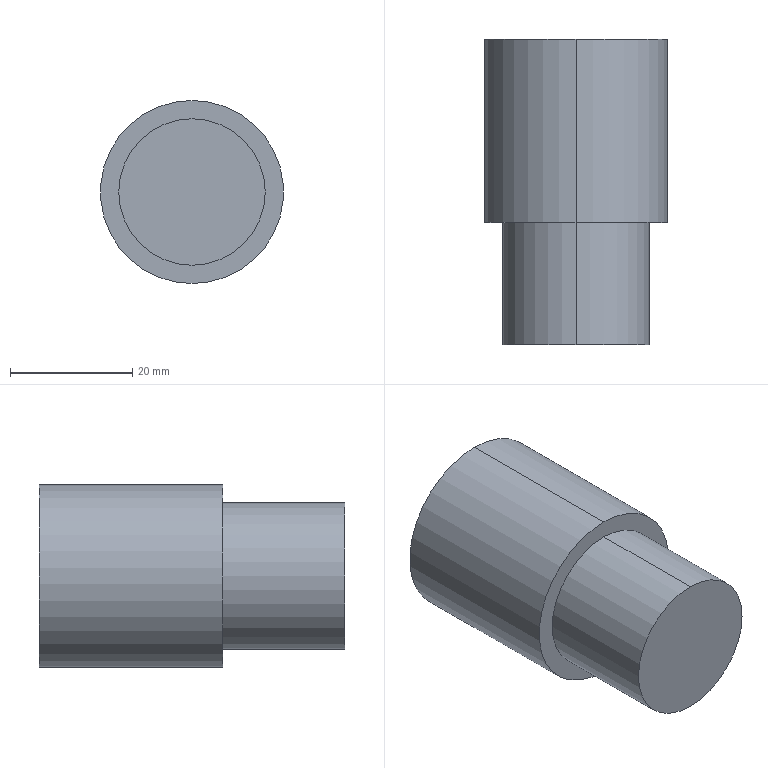Part | 1 solid | 13 faces | box 30 x 50 x 30 mm | volume 20948 mm3 | cylinder 8 | plane 5 | commonest cylinder face diameters 18 x2 20 x2 24 x2 30 x2
STEP:
#1=CARTESIAN_POINT('',(0.,-20.,-12.));
#2=VERTEX_POINT('',#1);
#3=CARTESIAN_POINT('',(0.,-20.,12.));
#4=VERTEX_POINT('',#3);
#5=CARTESIAN_POINT('',(0.,-20.,0.));
#6=DIRECTION('',(0.,-1.,0.));
#7=DIRECTION('',(0.,0.,-1.));
#8=AXIS2_PLACEMENT_3D('',#5,#6,#7);
#9=CIRCLE('',#8,12.);
#10=EDGE_CURVE('',#2,#4,#9,.T.);
#11=ORIENTED_EDGE('',*,*,#10,.F.);
#12=CARTESIAN_POINT('',(0.,0.,-12.));
#13=VERTEX_POINT('',#12);
#14=CARTESIAN_POINT('',(0.,-20.,-12.));
#15=DIRECTION('',(0.,1.,0.));
#16=VECTOR('',#15,1000.);
#17=LINE('',#14,#16);
#18=EDGE_CURVE('',#2,#13,#17,.T.);
#19=ORIENTED_EDGE('',*,*,#18,.T.);
#20=CARTESIAN_POINT('',(0.,0.,12.));
#21=VERTEX_POINT('',#20);
#22=CARTESIAN_POINT('',(0.,0.,0.));
#23=DIRECTION('',(0.,-1.,0.));
#24=DIRECTION('',(0.,0.,-1.));
#25=AXIS2_PLACEMENT_3D('',#22,#23,#24);
#26=CIRCLE('',#25,12.);
#27=EDGE_CURVE('',#13,#21,#26,.T.);
#28=ORIENTED_EDGE('',*,*,#27,.T.);
#29=CARTESIAN_POINT('',(0.,-20.,12.));
#30=DIRECTION('',(0.,1.,0.));
#31=VECTOR('',#30,1000.);
#32=LINE('',#29,#31);
#33=EDGE_CURVE('',#4,#21,#32,.T.);
#34=ORIENTED_EDGE('',*,*,#33,.F.);
#35=EDGE_LOOP('',(#11,#19,#28,#34));
#36=FACE_OUTER_BOUND('',#35,.T.);
#37=CARTESIAN_POINT('',(0.,-20.,0.));
#38=DIRECTION('',(0.,1.,0.));
#39=DIRECTION('',(0.,0.,1.));
#40=AXIS2_PLACEMENT_3D('',#37,#38,#39);
#41=CYLINDRICAL_SURFACE('',#40,12.);
#42=ADVANCED_FACE('',(#36),#41,.T.);
#43=CARTESIAN_POINT('',(0.,30.,15.));
#44=VERTEX_POINT('',#43);
#45=CARTESIAN_POINT('',(0.,30.,-15.));
#46=VERTEX_POINT('',#45);
#47=CARTESIAN_POINT('',(0.,30.,0.));
#48=DIRECTION('',(0.,1.,0.));
#49=DIRECTION('',(0.,0.,1.));
#50=AXIS2_PLACEMENT_3D('',#47,#48,#49);
#51=CIRCLE('',#50,15.);
#52=EDGE_CURVE('',#44,#46,#51,.T.);
#53=ORIENTED_EDGE('',*,*,#52,.F.);
#54=CARTESIAN_POINT('',(0.,0.,15.));
#55=VERTEX_POINT('',#54);
#56=CARTESIAN_POINT('',(0.,30.,15.));
#57=DIRECTION('',(0.,-1.,0.));
#58=VECTOR('',#57,1000.);
#59=LINE('',#56,#58);
#60=EDGE_CURVE('',#44,#55,#59,.T.);
#61=ORIENTED_EDGE('',*,*,#60,.T.);
#62=CARTESIAN_POINT('',(0.,0.,-15.));
#63=VERTEX_POINT('',#62);
#64=CARTESIAN_POINT('',(0.,0.,0.));
#65=DIRECTION('',(0.,1.,0.));
#66=DIRECTION('',(0.,0.,1.));
#67=AXIS2_PLACEMENT_3D('',#64,#65,#66);
#68=CIRCLE('',#67,15.);
#69=EDGE_CURVE('',#55,#63,#68,.T.);
#70=ORIENTED_EDGE('',*,*,#69,.T.);
#71=CARTESIAN_POINT('',(0.,30.,-15.));
#72=DIRECTION('',(0.,-1.,0.));
#73=VECTOR('',#72,1000.);
#74=LINE('',#71,#73);
#75=EDGE_CURVE('',#46,#63,#74,.T.);
#76=ORIENTED_EDGE('',*,*,#75,.F.);
#77=EDGE_LOOP('',(#53,#61,#70,#76));
#78=FACE_OUTER_BOUND('',#77,.T.);
#79=CARTESIAN_POINT('',(0.,30.,0.));
#80=DIRECTION('',(0.,-1.,0.));
#81=DIRECTION('',(0.,0.,-1.));
#82=AXIS2_PLACEMENT_3D('',#79,#80,#81);
#83=CYLINDRICAL_SURFACE('',#82,15.);
#84=ADVANCED_FACE('',(#78),#83,.T.);
#85=CARTESIAN_POINT('',(0.,28.,-9.));
#86=VERTEX_POINT('',#85);
#87=CARTESIAN_POINT('',(0.,28.,9.));
#88=VERTEX_POINT('',#87);
#89=CARTESIAN_POINT('',(0.,28.,0.));
#90=DIRECTION('',(0.,1.,0.));
#91=DIRECTION('',(0.,0.,1.));
#92=AXIS2_PLACEMENT_3D('',#89,#90,#91);
#93=CIRCLE('',#92,9.);
#94=EDGE_CURVE('',#86,#88,#93,.T.);
#95=ORIENTED_EDGE('',*,*,#94,.F.);
#96=CARTESIAN_POINT('',(0.,30.,-9.));
#97=VERTEX_POINT('',#96);
#98=CARTESIAN_POINT('',(0.,25.,-9.));
#99=DIRECTION('',(0.,1.,0.));
#100=VECTOR('',#99,1000.);
#101=LINE('',#98,#100);
#102=EDGE_CURVE('',#86,#97,#101,.T.);
#103=ORIENTED_EDGE('',*,*,#102,.T.);
#104=CARTESIAN_POINT('',(0.,30.,9.));
#105=VERTEX_POINT('',#104);
#106=CARTESIAN_POINT('',(0.,30.,0.));
#107=DIRECTION('',(0.,1.,0.));
#108=DIRECTION('',(0.,0.,1.));
#109=AXIS2_PLACEMENT_3D('',#106,#107,#108);
#110=CIRCLE('',#109,9.);
#111=EDGE_CURVE('',#97,#105,#110,.T.);
#112=ORIENTED_EDGE('',*,*,#111,.T.);
#113=CARTESIAN_POINT('',(0.,25.,9.));
#114=DIRECTION('',(0.,1.,0.));
#115=VECTOR('',#114,1000.);
#116=LINE('',#113,#115);
#117=EDGE_CURVE('',#88,#105,#116,.T.);
#118=ORIENTED_EDGE('',*,*,#117,.F.);
#119=EDGE_LOOP('',(#95,#103,#112,#118));
#120=FACE_OUTER_BOUND('',#119,.T.);
#121=CARTESIAN_POINT('',(0.,25.,0.));
#122=DIRECTION('',(0.,1.,0.));
#123=DIRECTION('',(0.,0.,1.));
#124=AXIS2_PLACEMENT_3D('',#121,#122,#123);
#125=CYLINDRICAL_SURFACE('',#124,9.);
#126=ADVANCED_FACE('',(#120),#125,.F.);
#127=CARTESIAN_POINT('',(0.,0.,-10.));
#128=VERTEX_POINT('',#127);
#129=CARTESIAN_POINT('',(0.,0.,10.));
#130=VERTEX_POINT('',#129);
#131=CARTESIAN_POINT('',(0.,0.,0.));
#132=DIRECTION('',(0.,1.,0.));
#133=DIRECTION('',(0.,0.,1.));
#134=AXIS2_PLACEMENT_3D('',#131,#132,#133);
#135=CIRCLE('',#134,10.);
#136=EDGE_CURVE('',#128,#130,#135,.T.);
#137=ORIENTED_EDGE('',*,*,#136,.F.);
#138=CARTESIAN_POINT('',(0.,28.,-10.));
#139=VERTEX_POINT('',#138);
#140=CARTESIAN_POINT('',(0.,0.,-10.));
#141=DIRECTION('',(0.,1.,0.));
#142=VECTOR('',#141,1000.);
#143=LINE('',#140,#142);
#144=EDGE_CURVE('',#128,#139,#143,.T.);
#145=ORIENTED_EDGE('',*,*,#144,.T.);
#146=CARTESIAN_POINT('',(0.,28.,10.));
#147=VERTEX_POINT('',#146);
#148=CARTESIAN_POINT('',(0.,28.,0.));
#149=DIRECTION('',(0.,1.,0.));
#150=DIRECTION('',(0.,0.,1.));
#151=AXIS2_PLACEMENT_3D('',#148,#149,#150);
#152=CIRCLE('',#151,10.);
#153=EDGE_CURVE('',#139,#147,#152,.T.);
#154=ORIENTED_EDGE('',*,*,#153,.T.);
#155=CARTESIAN_POINT('',(0.,0.,10.));
#156=DIRECTION('',(0.,1.,0.));
#157=VECTOR('',#156,1000.);
#158=LINE('',#155,#157);
#159=EDGE_CURVE('',#130,#147,#158,.T.);
#160=ORIENTED_EDGE('',*,*,#159,.F.);
#161=EDGE_LOOP('',(#137,#145,#154,#160));
#162=FACE_OUTER_BOUND('',#161,.T.);
#163=CARTESIAN_POINT('',(0.,0.,0.));
#164=DIRECTION('',(0.,1.,0.));
#165=DIRECTION('',(0.,0.,1.));
#166=AXIS2_PLACEMENT_3D('',#163,#164,#165);
#167=CYLINDRICAL_SURFACE('',#166,10.);
#168=ADVANCED_FACE('',(#162),#167,.F.);
#169=ORIENTED_EDGE('',*,*,#144,.F.);
#170=CARTESIAN_POINT('',(0.,0.,0.));
#171=DIRECTION('',(0.,1.,0.));
#172=DIRECTION('',(0.,0.,1.));
#173=AXIS2_PLACEMENT_3D('',#170,#171,#172);
#174=CIRCLE('',#173,10.);
#175=EDGE_CURVE('',#130,#128,#174,.T.);
#176=ORIENTED_EDGE('',*,*,#175,.F.);
#177=ORIENTED_EDGE('',*,*,#159,.T.);
#178=CARTESIAN_POINT('',(0.,28.,0.));
#179=DIRECTION('',(0.,1.,0.));
#180=DIRECTION('',(0.,0.,1.));
#181=AXIS2_PLACEMENT_3D('',#178,#179,#180);
#182=CIRCLE('',#181,10.);
#183=EDGE_CURVE('',#147,#139,#182,.T.);
#184=ORIENTED_EDGE('',*,*,#183,.T.);
#185=EDGE_LOOP('',(#169,#176,#177,#184));
#186=FACE_OUTER_BOUND('',#185,.T.);
#187=CARTESIAN_POINT('',(0.,0.,0.));
#188=DIRECTION('',(0.,1.,0.));
#189=DIRECTION('',(0.,0.,1.));
#190=AXIS2_PLACEMENT_3D('',#187,#188,#189);
#191=CYLINDRICAL_SURFACE('',#190,10.);
#192=ADVANCED_FACE('',(#186),#191,.F.);
#193=ORIENTED_EDGE('',*,*,#175,.T.);
#194=ORIENTED_EDGE('',*,*,#136,.T.);
#195=EDGE_LOOP('',(#193,#194));
#196=FACE_OUTER_BOUND('',#195,.T.);
#197=CARTESIAN_POINT('',(0.,0.,0.));
#198=DIRECTION('',(0.,1.,0.));
#199=DIRECTION('',(0.,0.,1.));
#200=AXIS2_PLACEMENT_3D('',#197,#198,#199);
#201=PLANE('',#200);
#202=ADVANCED_FACE('',(#196),#201,.T.);
#203=CARTESIAN_POINT('',(0.,28.,0.));
#204=DIRECTION('',(0.,1.,0.));
#205=DIRECTION('',(0.,0.,1.));
#206=AXIS2_PLACEMENT_3D('',#203,#204,#205);
#207=CIRCLE('',#206,9.);
#208=EDGE_CURVE('',#88,#86,#207,.T.);
#209=ORIENTED_EDGE('',*,*,#208,.T.);
#210=ORIENTED_EDGE('',*,*,#94,.T.);
#211=EDGE_LOOP('',(#209,#210));
#212=FACE_BOUND('',#211,.T.);
#213=ORIENTED_EDGE('',*,*,#183,.F.);
#214=ORIENTED_EDGE('',*,*,#153,.F.);
#215=EDGE_LOOP('',(#213,#214));
#216=FACE_OUTER_BOUND('',#215,.T.);
#217=CARTESIAN_POINT('',(0.,28.,0.));
#218=DIRECTION('',(0.,1.,0.));
#219=DIRECTION('',(0.,0.,1.));
#220=AXIS2_PLACEMENT_3D('',#217,#218,#219);
#221=PLANE('',#220);
#222=ADVANCED_FACE('',(#212,#216),#221,.F.);
#223=ORIENTED_EDGE('',*,*,#102,.F.);
#224=ORIENTED_EDGE('',*,*,#208,.F.);
#225=ORIENTED_EDGE('',*,*,#117,.T.);
#226=CARTESIAN_POINT('',(0.,30.,0.));
#227=DIRECTION('',(0.,1.,0.));
#228=DIRECTION('',(0.,0.,1.));
#229=AXIS2_PLACEMENT_3D('',#226,#227,#228);
#230=CIRCLE('',#229,9.);
#231=EDGE_CURVE('',#105,#97,#230,.T.);
#232=ORIENTED_EDGE('',*,*,#231,.T.);
#233=EDGE_LOOP('',(#223,#224,#225,#232));
#234=FACE_OUTER_BOUND('',#233,.T.);
#235=CARTESIAN_POINT('',(0.,25.,0.));
#236=DIRECTION('',(0.,1.,0.));
#237=DIRECTION('',(0.,0.,1.));
#238=AXIS2_PLACEMENT_3D('',#235,#236,#237);
#239=CYLINDRICAL_SURFACE('',#238,9.);
#240=ADVANCED_FACE('',(#234),#239,.F.);
#241=ORIENTED_EDGE('',*,*,#60,.F.);
#242=CARTESIAN_POINT('',(0.,30.,0.));
#243=DIRECTION('',(0.,1.,0.));
#244=DIRECTION('',(0.,0.,1.));
#245=AXIS2_PLACEMENT_3D('',#242,#243,#244);
#246=CIRCLE('',#245,15.);
#247=EDGE_CURVE('',#46,#44,#246,.T.);
#248=ORIENTED_EDGE('',*,*,#247,.F.);
#249=ORIENTED_EDGE('',*,*,#75,.T.);
#250=CARTESIAN_POINT('',(0.,0.,0.));
#251=DIRECTION('',(0.,1.,0.));
#252=DIRECTION('',(0.,0.,1.));
#253=AXIS2_PLACEMENT_3D('',#250,#251,#252);
#254=CIRCLE('',#253,15.);
#255=EDGE_CURVE('',#63,#55,#254,.T.);
#256=ORIENTED_EDGE('',*,*,#255,.T.);
#257=EDGE_LOOP('',(#241,#248,#249,#256));
#258=FACE_OUTER_BOUND('',#257,.T.);
#259=CARTESIAN_POINT('',(0.,30.,0.));
#260=DIRECTION('',(0.,-1.,0.));
#261=DIRECTION('',(0.,0.,-1.));
#262=AXIS2_PLACEMENT_3D('',#259,#260,#261);
#263=CYLINDRICAL_SURFACE('',#262,15.);
#264=ADVANCED_FACE('',(#258),#263,.T.);
#265=ORIENTED_EDGE('',*,*,#231,.F.);
#266=ORIENTED_EDGE('',*,*,#111,.F.);
#267=EDGE_LOOP('',(#265,#266));
#268=FACE_BOUND('',#267,.T.);
#269=ORIENTED_EDGE('',*,*,#247,.T.);
#270=ORIENTED_EDGE('',*,*,#52,.T.);
#271=EDGE_LOOP('',(#269,#270));
#272=FACE_OUTER_BOUND('',#271,.T.);
#273=CARTESIAN_POINT('',(0.,30.,0.));
#274=DIRECTION('',(0.,1.,0.));
#275=DIRECTION('',(0.,0.,1.));
#276=AXIS2_PLACEMENT_3D('',#273,#274,#275);
#277=PLANE('',#276);
#278=ADVANCED_FACE('',(#268,#272),#277,.T.);
#279=CARTESIAN_POINT('',(0.,0.,0.));
#280=DIRECTION('',(0.,-1.,0.));
#281=DIRECTION('',(0.,0.,-1.));
#282=AXIS2_PLACEMENT_3D('',#279,#280,#281);
#283=CIRCLE('',#282,12.);
#284=EDGE_CURVE('',#21,#13,#283,.T.);
#285=ORIENTED_EDGE('',*,*,#284,.F.);
#286=ORIENTED_EDGE('',*,*,#27,.F.);
#287=EDGE_LOOP('',(#285,#286));
#288=FACE_BOUND('',#287,.T.);
#289=ORIENTED_EDGE('',*,*,#255,.F.);
#290=ORIENTED_EDGE('',*,*,#69,.F.);
#291=EDGE_LOOP('',(#289,#290));
#292=FACE_OUTER_BOUND('',#291,.T.);
#293=CARTESIAN_POINT('',(0.,0.,0.));
#294=DIRECTION('',(0.,1.,0.));
#295=DIRECTION('',(0.,0.,1.));
#296=AXIS2_PLACEMENT_3D('',#293,#294,#295);
#297=PLANE('',#296);
#298=ADVANCED_FACE('',(#288,#292),#297,.F.);
#299=ORIENTED_EDGE('',*,*,#18,.F.);
#300=CARTESIAN_POINT('',(0.,-20.,0.));
#301=DIRECTION('',(0.,-1.,0.));
#302=DIRECTION('',(0.,0.,-1.));
#303=AXIS2_PLACEMENT_3D('',#300,#301,#302);
#304=CIRCLE('',#303,12.);
#305=EDGE_CURVE('',#4,#2,#304,.T.);
#306=ORIENTED_EDGE('',*,*,#305,.F.);
#307=ORIENTED_EDGE('',*,*,#33,.T.);
#308=ORIENTED_EDGE('',*,*,#284,.T.);
#309=EDGE_LOOP('',(#299,#306,#307,#308));
#310=FACE_OUTER_BOUND('',#309,.T.);
#311=CARTESIAN_POINT('',(0.,-20.,0.));
#312=DIRECTION('',(0.,1.,0.));
#313=DIRECTION('',(0.,0.,1.));
#314=AXIS2_PLACEMENT_3D('',#311,#312,#313);
#315=CYLINDRICAL_SURFACE('',#314,12.);
#316=ADVANCED_FACE('',(#310),#315,.T.);
#317=ORIENTED_EDGE('',*,*,#305,.T.);
#318=ORIENTED_EDGE('',*,*,#10,.T.);
#319=EDGE_LOOP('',(#317,#318));
#320=FACE_OUTER_BOUND('',#319,.T.);
#321=CARTESIAN_POINT('',(0.,-20.,0.));
#322=DIRECTION('',(0.,-1.,0.));
#323=DIRECTION('',(0.,0.,-1.));
#324=AXIS2_PLACEMENT_3D('',#321,#322,#323);
#325=PLANE('',#324);
#326=ADVANCED_FACE('',(#320),#325,.T.);
#327=CLOSED_SHELL('',(#42,#84,#126,#168,#192,#202,#222,#240,#264,#278,#298,#316,#326));
#328=MANIFOLD_SOLID_BREP('',#327);
#329=CARTESIAN_POINT('',(0.,0.,0.));
#330=DIRECTION('',(0.,0.,1.));
#331=DIRECTION('',(1.,0.,0.));
#332=AXIS2_PLACEMENT_3D('',#329,#330,#331);
#333=(LENGTH_UNIT()NAMED_UNIT(*)SI_UNIT(.MILLI.,.METRE.));
#334=UNCERTAINTY_MEASURE_WITH_UNIT(LENGTH_MEASURE(0.00001),#333,'','');
#335=(NAMED_UNIT(*)PLANE_ANGLE_UNIT()SI_UNIT($,.RADIAN.));
#336=(NAMED_UNIT(*)SI_UNIT($,.STERADIAN.)SOLID_ANGLE_UNIT());
#337=(GEOMETRIC_REPRESENTATION_CONTEXT(3)GLOBAL_UNCERTAINTY_ASSIGNED_CONTEXT((#334))GLOBAL_UNIT_ASSIGNED_CONTEXT((#333,#335,#336))REPRESENTATION_CONTEXT('',''));
#338=ADVANCED_BREP_SHAPE_REPRESENTATION('',(#328,#332),#337);